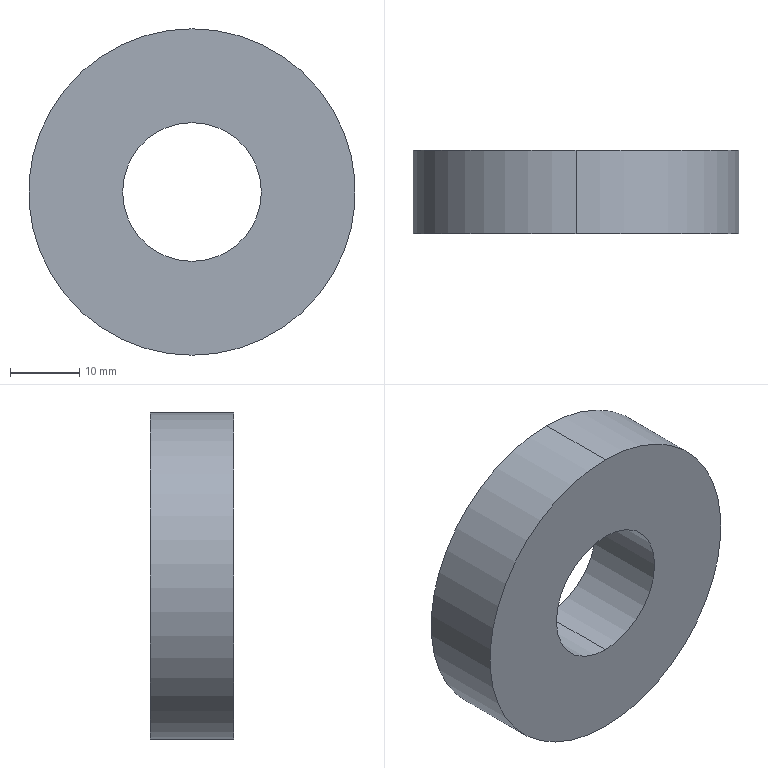Part | SolidWorks | features Extrusion 1 | 1 solid | 6 faces | box 47 x 12 x 47 mm | volume 17049 mm3 | cylinder 4 | plane 2 | commonest cylinder face diameters 20 x2 47 x2
STEP:
#1=CARTESIAN_POINT('',(0.,12.,-10.));
#2=VERTEX_POINT('',#1);
#3=CARTESIAN_POINT('',(0.,12.,10.));
#4=VERTEX_POINT('',#3);
#5=CARTESIAN_POINT('',(0.,12.,0.));
#6=DIRECTION('',(0.,1.,0.));
#7=DIRECTION('',(0.,0.,1.));
#8=AXIS2_PLACEMENT_3D('',#5,#6,#7);
#9=CIRCLE('',#8,10.);
#10=EDGE_CURVE('',#2,#4,#9,.T.);
#11=ORIENTED_EDGE('',*,*,#10,.T.);
#12=CARTESIAN_POINT('',(0.,0.,10.));
#13=VERTEX_POINT('',#12);
#14=CARTESIAN_POINT('',(0.,12.,10.));
#15=DIRECTION('',(0.,-1.,0.));
#16=VECTOR('',#15,1000.);
#17=LINE('',#14,#16);
#18=EDGE_CURVE('',#4,#13,#17,.T.);
#19=ORIENTED_EDGE('',*,*,#18,.T.);
#20=CARTESIAN_POINT('',(0.,0.,-10.));
#21=VERTEX_POINT('',#20);
#22=CARTESIAN_POINT('',(0.,0.,0.));
#23=DIRECTION('',(0.,1.,0.));
#24=DIRECTION('',(0.,0.,1.));
#25=AXIS2_PLACEMENT_3D('',#22,#23,#24);
#26=CIRCLE('',#25,10.);
#27=EDGE_CURVE('',#21,#13,#26,.T.);
#28=ORIENTED_EDGE('',*,*,#27,.F.);
#29=CARTESIAN_POINT('',(0.,12.,-10.));
#30=DIRECTION('',(0.,-1.,0.));
#31=VECTOR('',#30,1000.);
#32=LINE('',#29,#31);
#33=EDGE_CURVE('',#2,#21,#32,.T.);
#34=ORIENTED_EDGE('',*,*,#33,.F.);
#35=EDGE_LOOP('',(#11,#19,#28,#34));
#36=FACE_OUTER_BOUND('',#35,.T.);
#37=CARTESIAN_POINT('',(0.,12.,0.));
#38=DIRECTION('',(0.,-1.,0.));
#39=DIRECTION('',(0.,0.,-1.));
#40=AXIS2_PLACEMENT_3D('',#37,#38,#39);
#41=CYLINDRICAL_SURFACE('',#40,10.);
#42=ADVANCED_FACE('',(#36),#41,.F.);
#43=CARTESIAN_POINT('',(0.,12.,23.5));
#44=VERTEX_POINT('',#43);
#45=CARTESIAN_POINT('',(0.,12.,-23.5));
#46=VERTEX_POINT('',#45);
#47=CARTESIAN_POINT('',(0.,12.,0.));
#48=DIRECTION('',(0.,1.,0.));
#49=DIRECTION('',(0.,0.,1.));
#50=AXIS2_PLACEMENT_3D('',#47,#48,#49);
#51=CIRCLE('',#50,23.5);
#52=EDGE_CURVE('',#44,#46,#51,.T.);
#53=ORIENTED_EDGE('',*,*,#52,.F.);
#54=CARTESIAN_POINT('',(0.,0.,23.5));
#55=VERTEX_POINT('',#54);
#56=CARTESIAN_POINT('',(0.,12.,23.5));
#57=DIRECTION('',(0.,-1.,0.));
#58=VECTOR('',#57,1000.);
#59=LINE('',#56,#58);
#60=EDGE_CURVE('',#44,#55,#59,.T.);
#61=ORIENTED_EDGE('',*,*,#60,.T.);
#62=CARTESIAN_POINT('',(0.,0.,-23.5));
#63=VERTEX_POINT('',#62);
#64=CARTESIAN_POINT('',(0.,0.,0.));
#65=DIRECTION('',(0.,1.,0.));
#66=DIRECTION('',(0.,0.,1.));
#67=AXIS2_PLACEMENT_3D('',#64,#65,#66);
#68=CIRCLE('',#67,23.5);
#69=EDGE_CURVE('',#55,#63,#68,.T.);
#70=ORIENTED_EDGE('',*,*,#69,.T.);
#71=CARTESIAN_POINT('',(0.,12.,-23.5));
#72=DIRECTION('',(0.,-1.,0.));
#73=VECTOR('',#72,1000.);
#74=LINE('',#71,#73);
#75=EDGE_CURVE('',#46,#63,#74,.T.);
#76=ORIENTED_EDGE('',*,*,#75,.F.);
#77=EDGE_LOOP('',(#53,#61,#70,#76));
#78=FACE_OUTER_BOUND('',#77,.T.);
#79=CARTESIAN_POINT('',(0.,12.,0.));
#80=DIRECTION('',(0.,-1.,0.));
#81=DIRECTION('',(0.,0.,-1.));
#82=AXIS2_PLACEMENT_3D('',#79,#80,#81);
#83=CYLINDRICAL_SURFACE('',#82,23.5);
#84=ADVANCED_FACE('',(#78),#83,.T.);
#85=CARTESIAN_POINT('',(0.,12.,0.));
#86=DIRECTION('',(0.,1.,0.));
#87=DIRECTION('',(0.,0.,1.));
#88=AXIS2_PLACEMENT_3D('',#85,#86,#87);
#89=CIRCLE('',#88,23.5);
#90=EDGE_CURVE('',#46,#44,#89,.T.);
#91=ORIENTED_EDGE('',*,*,#90,.T.);
#92=ORIENTED_EDGE('',*,*,#52,.T.);
#93=EDGE_LOOP('',(#91,#92));
#94=FACE_OUTER_BOUND('',#93,.T.);
#95=ORIENTED_EDGE('',*,*,#10,.F.);
#96=CARTESIAN_POINT('',(0.,12.,0.));
#97=DIRECTION('',(0.,1.,0.));
#98=DIRECTION('',(0.,0.,1.));
#99=AXIS2_PLACEMENT_3D('',#96,#97,#98);
#100=CIRCLE('',#99,10.);
#101=EDGE_CURVE('',#4,#2,#100,.T.);
#102=ORIENTED_EDGE('',*,*,#101,.F.);
#103=EDGE_LOOP('',(#95,#102));
#104=FACE_BOUND('',#103,.T.);
#105=CARTESIAN_POINT('',(0.,12.,0.));
#106=DIRECTION('',(0.,1.,0.));
#107=DIRECTION('',(0.,0.,1.));
#108=AXIS2_PLACEMENT_3D('',#105,#106,#107);
#109=PLANE('',#108);
#110=ADVANCED_FACE('',(#94,#104),#109,.T.);
#111=CARTESIAN_POINT('',(0.,0.,0.));
#112=DIRECTION('',(0.,1.,0.));
#113=DIRECTION('',(0.,0.,1.));
#114=AXIS2_PLACEMENT_3D('',#111,#112,#113);
#115=CIRCLE('',#114,23.5);
#116=EDGE_CURVE('',#63,#55,#115,.T.);
#117=ORIENTED_EDGE('',*,*,#116,.F.);
#118=ORIENTED_EDGE('',*,*,#69,.F.);
#119=EDGE_LOOP('',(#117,#118));
#120=FACE_OUTER_BOUND('',#119,.T.);
#121=ORIENTED_EDGE('',*,*,#27,.T.);
#122=CARTESIAN_POINT('',(0.,0.,0.));
#123=DIRECTION('',(0.,1.,0.));
#124=DIRECTION('',(0.,0.,1.));
#125=AXIS2_PLACEMENT_3D('',#122,#123,#124);
#126=CIRCLE('',#125,10.);
#127=EDGE_CURVE('',#13,#21,#126,.T.);
#128=ORIENTED_EDGE('',*,*,#127,.T.);
#129=EDGE_LOOP('',(#121,#128));
#130=FACE_BOUND('',#129,.T.);
#131=CARTESIAN_POINT('',(0.,0.,0.));
#132=DIRECTION('',(0.,1.,0.));
#133=DIRECTION('',(0.,0.,1.));
#134=AXIS2_PLACEMENT_3D('',#131,#132,#133);
#135=PLANE('',#134);
#136=ADVANCED_FACE('',(#120,#130),#135,.F.);
#137=ORIENTED_EDGE('',*,*,#60,.F.);
#138=ORIENTED_EDGE('',*,*,#90,.F.);
#139=ORIENTED_EDGE('',*,*,#75,.T.);
#140=ORIENTED_EDGE('',*,*,#116,.T.);
#141=EDGE_LOOP('',(#137,#138,#139,#140));
#142=FACE_OUTER_BOUND('',#141,.T.);
#143=CARTESIAN_POINT('',(0.,12.,0.));
#144=DIRECTION('',(0.,-1.,0.));
#145=DIRECTION('',(0.,0.,-1.));
#146=AXIS2_PLACEMENT_3D('',#143,#144,#145);
#147=CYLINDRICAL_SURFACE('',#146,23.5);
#148=ADVANCED_FACE('',(#142),#147,.T.);
#149=ORIENTED_EDGE('',*,*,#18,.F.);
#150=ORIENTED_EDGE('',*,*,#101,.T.);
#151=ORIENTED_EDGE('',*,*,#33,.T.);
#152=ORIENTED_EDGE('',*,*,#127,.F.);
#153=EDGE_LOOP('',(#149,#150,#151,#152));
#154=FACE_OUTER_BOUND('',#153,.T.);
#155=CARTESIAN_POINT('',(0.,12.,0.));
#156=DIRECTION('',(0.,-1.,0.));
#157=DIRECTION('',(0.,0.,-1.));
#158=AXIS2_PLACEMENT_3D('',#155,#156,#157);
#159=CYLINDRICAL_SURFACE('',#158,10.);
#160=ADVANCED_FACE('',(#154),#159,.F.);
#161=CLOSED_SHELL('',(#42,#84,#110,#136,#148,#160));
#162=MANIFOLD_SOLID_BREP('',#161);
#163=CARTESIAN_POINT('',(0.,0.,0.));
#164=DIRECTION('',(0.,0.,1.));
#165=DIRECTION('',(1.,0.,0.));
#166=AXIS2_PLACEMENT_3D('',#163,#164,#165);
#167=(LENGTH_UNIT()NAMED_UNIT(*)SI_UNIT(.MILLI.,.METRE.));
#168=UNCERTAINTY_MEASURE_WITH_UNIT(LENGTH_MEASURE(0.00001),#167,'','');
#169=(NAMED_UNIT(*)PLANE_ANGLE_UNIT()SI_UNIT($,.RADIAN.));
#170=(NAMED_UNIT(*)SI_UNIT($,.STERADIAN.)SOLID_ANGLE_UNIT());
#171=(GEOMETRIC_REPRESENTATION_CONTEXT(3)GLOBAL_UNCERTAINTY_ASSIGNED_CONTEXT((#168))GLOBAL_UNIT_ASSIGNED_CONTEXT((#167,#169,#170))REPRESENTATION_CONTEXT('',''));
#172=ADVANCED_BREP_SHAPE_REPRESENTATION('',(#162,#166),#171);